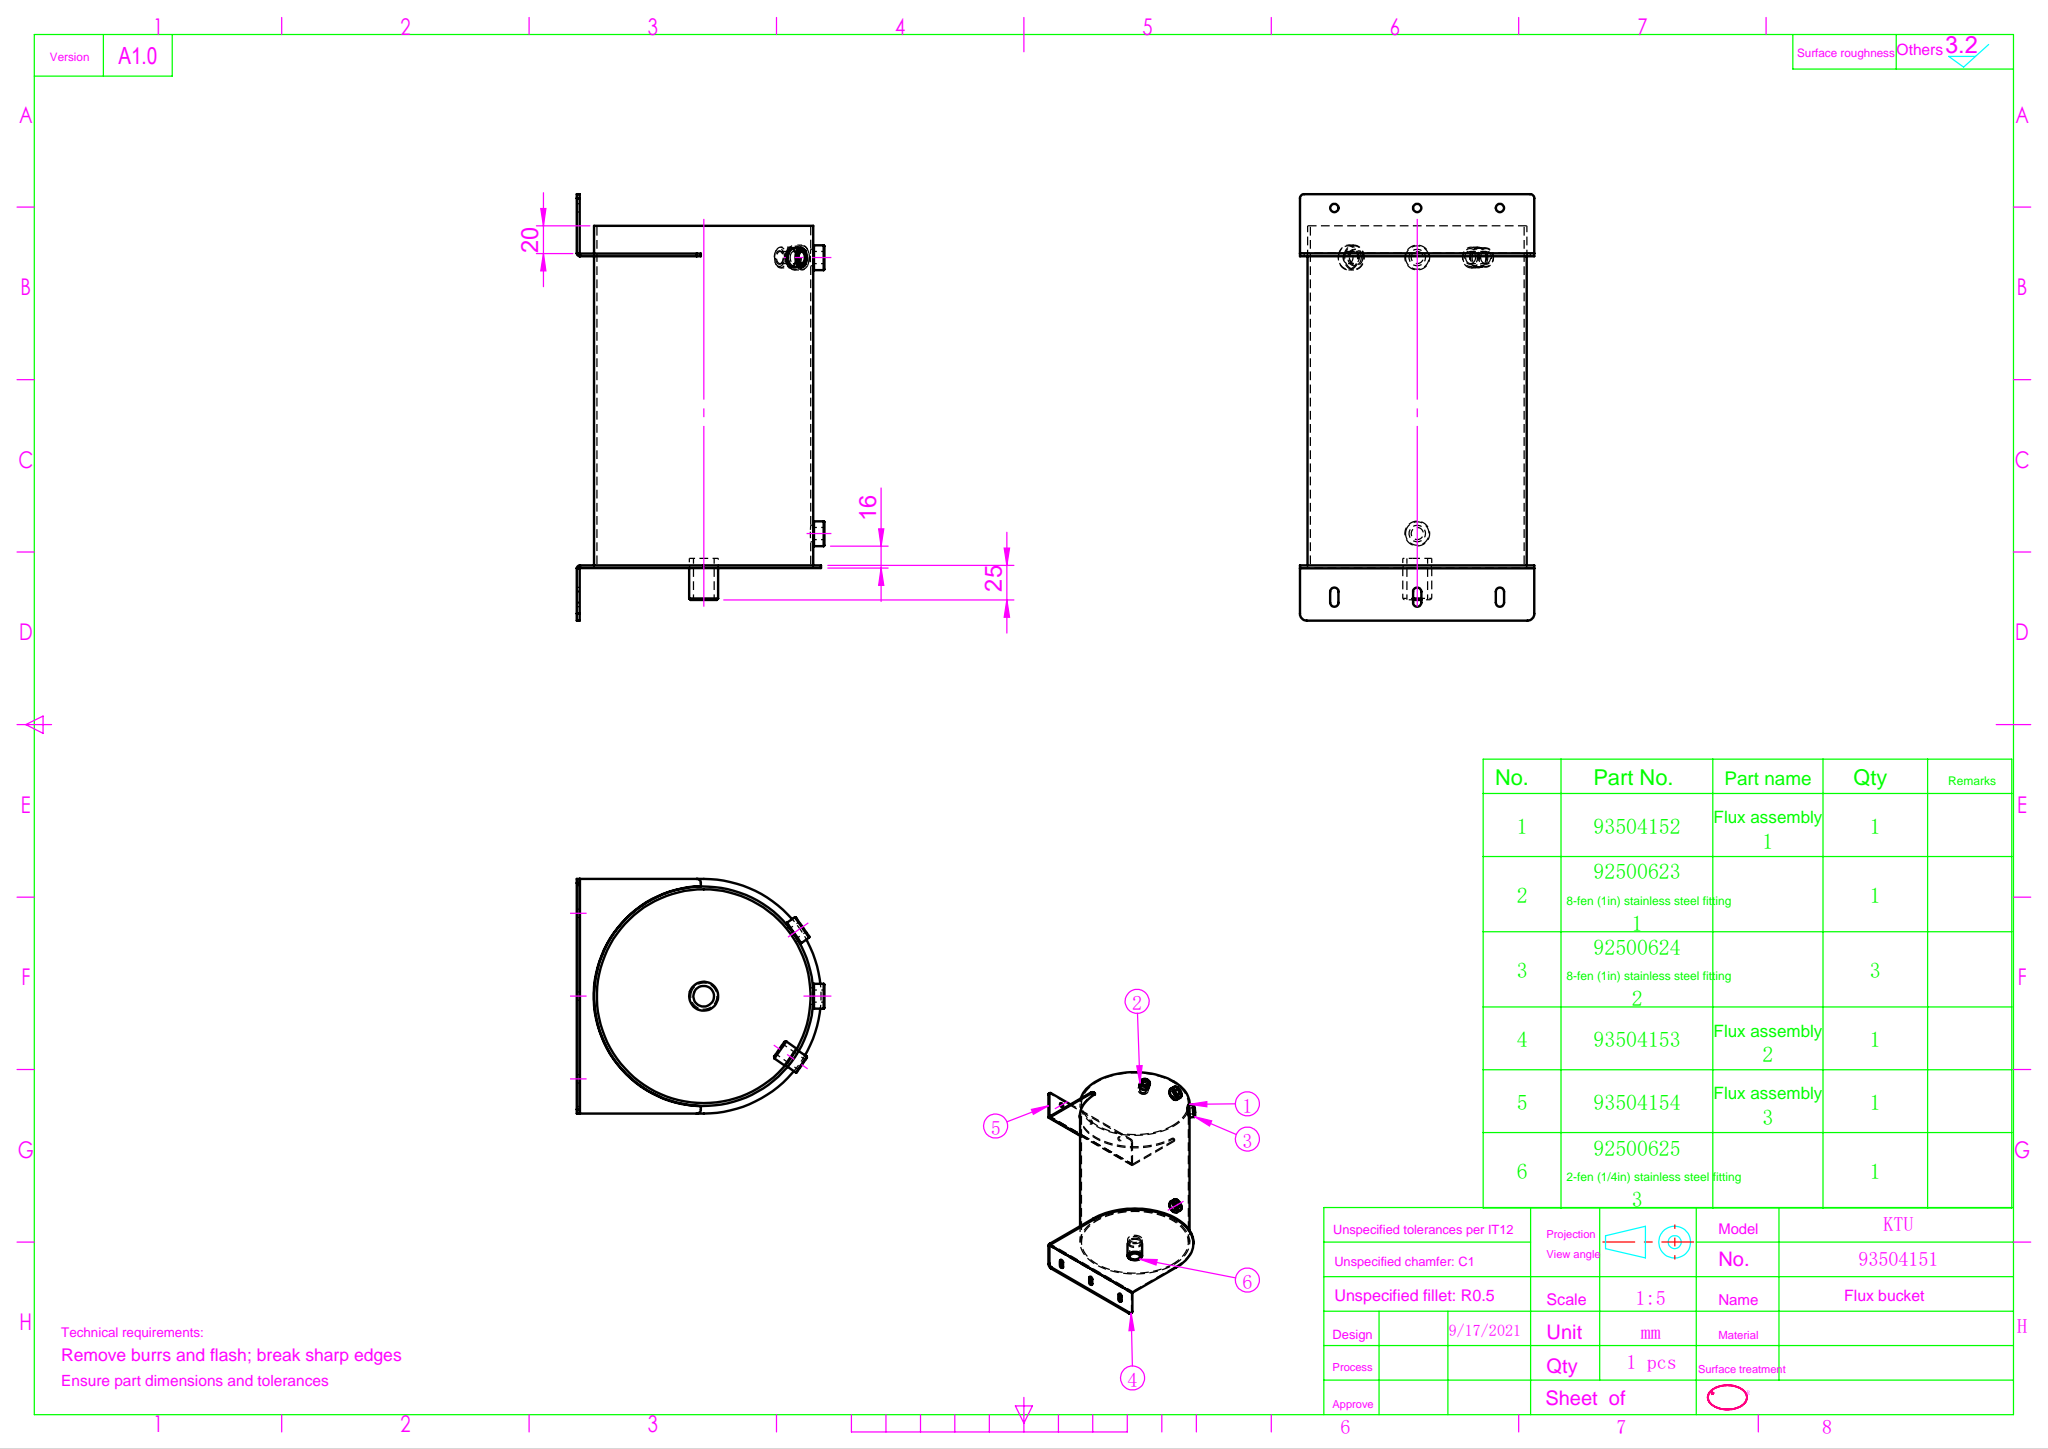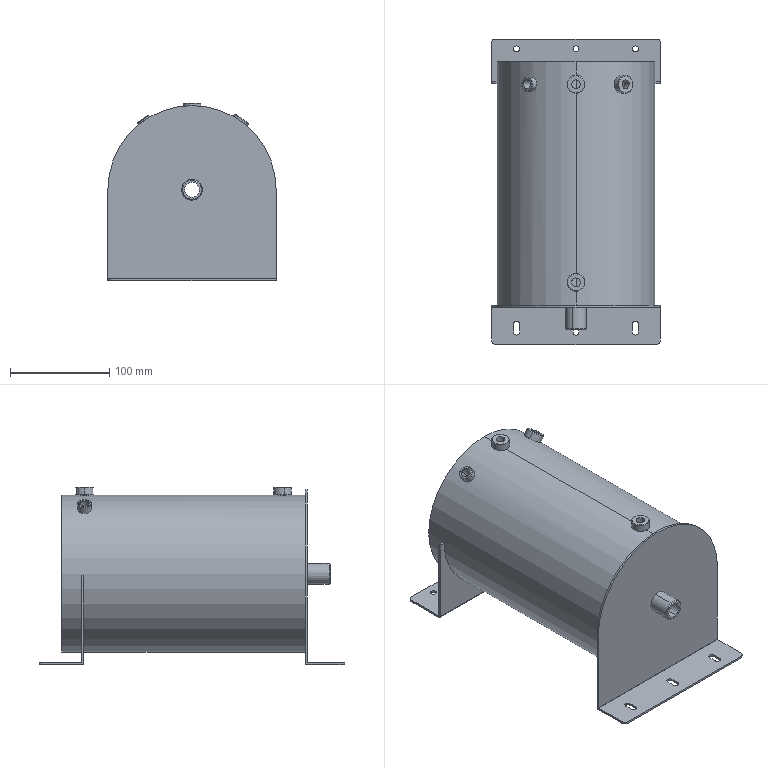Part | SolidWorks | 8 solids | 126 faces | box 170 x 309 x 179.5 mm | volume 344501 mm3 | cylinder 61 | plane 43 | cone 22 | commonest cylinder face diameters 6 x16 8.8 x8 12 x6 18 x6 14 x4 15 x4